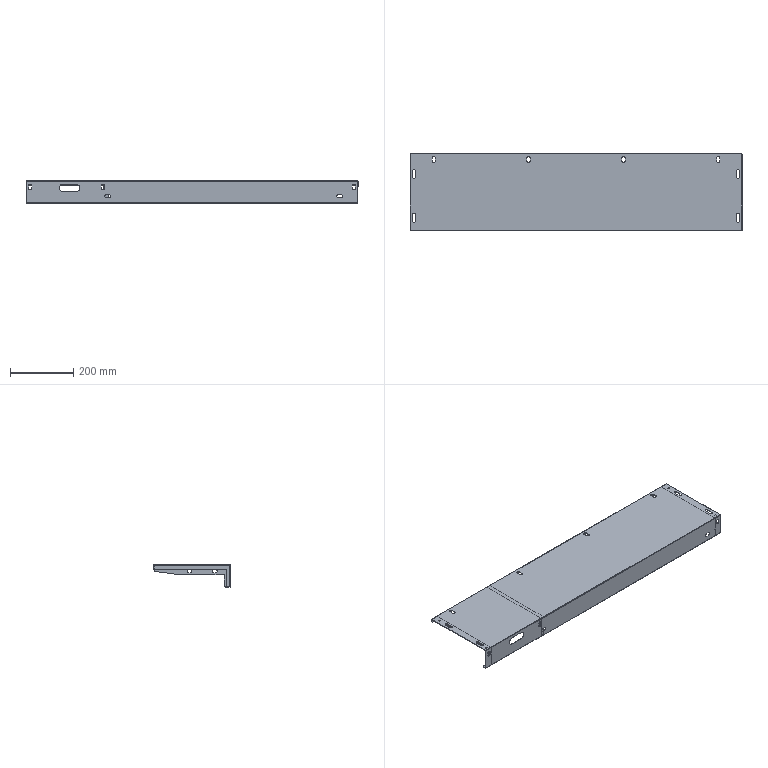Part | 4 solids | 214 faces | box 1050 x 243.5 x 70 mm | volume 464192 mm3 | plane 133 | cylinder 81 | commonest cylinder face diameters 10 x24 9 x20 6 x10 11 x8 0.4 x7 2.4 x4